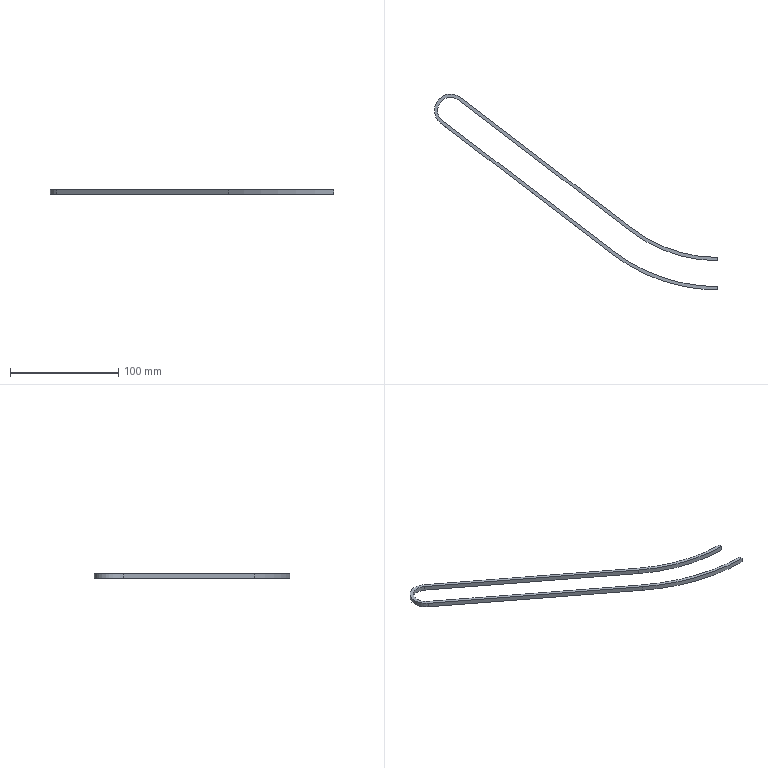Part | STEP file | 1 solid | 15 faces | box 261.956 x 181.154 x 4 mm | volume 7579 mm3 | plane 8 | cylinder 7 | commonest cylinder face diameters 24 x2 30 x1 260 x1 266 x1 314 x1 320 x1
STEP:
#1=CARTESIAN_POINT('',(0.,0.,0.));
#2=DIRECTION('',(0.,0.,1.));
#3=DIRECTION('',(1.,0.,0.));
#4=AXIS2_PLACEMENT_3D('',#1,#2,#3);
#5=CARTESIAN_POINT('',(-78.156,99.707,0.));
#6=VERTEX_POINT('',#5);
#7=CARTESIAN_POINT('',(-78.156,99.707,4.));
#8=VERTEX_POINT('',#7);
#9=CARTESIAN_POINT('',(-78.156,99.707,4.));
#10=DIRECTION('',(0.,0.,1.));
#11=VECTOR('',#10,1.);
#12=LINE('',#9,#11);
#13=CARTESIAN_POINT('',(-85.439,90.17,4.));
#14=DIRECTION('',(0.,0.,-1.));
#15=DIRECTION('',(-1.,0.,0.));
#16=AXIS2_PLACEMENT_3D('',#13,#14,#15);
#17=CYLINDRICAL_SURFACE('',#16,12.);
#18=CARTESIAN_POINT('',(2.223,0.));
#19=DIRECTION('',(0.,-1.));
#20=VECTOR('',#19,1.);
#21=LINE('',#18,#20);
#22=(GEOMETRIC_REPRESENTATION_CONTEXT(2)PARAMETRIC_REPRESENTATION_CONTEXT()REPRESENTATION_CONTEXT('',''));
#23=DEFINITIONAL_REPRESENTATION('',(#21),#22);
#24=PCURVE('',#17,#23);
#25=CARTESIAN_POINT('',(-78.156,99.707,4.));
#26=DIRECTION('',(0.607,0.7947,0.));
#27=DIRECTION('',(-0.7947,0.607,0.));
#28=AXIS2_PLACEMENT_3D('',#25,#26,#27);
#29=PLANE('',#28);
#30=CARTESIAN_POINT('',(0.,0.));
#31=DIRECTION('',(0.,1.));
#32=VECTOR('',#31,1.);
#33=LINE('',#30,#32);
#34=(GEOMETRIC_REPRESENTATION_CONTEXT(2)PARAMETRIC_REPRESENTATION_CONTEXT()REPRESENTATION_CONTEXT('',''));
#35=DEFINITIONAL_REPRESENTATION('',(#33),#34);
#36=PCURVE('',#29,#35);
#37=SURFACE_CURVE('',#12,(#24,#36),.PCURVE_S1.);
#38=EDGE_CURVE('',#6,#8,#37,.T.);
#39=ORIENTED_EDGE('',*,*,#38,.F.);
#40=CARTESIAN_POINT('',(-97.439,90.17,0.));
#41=VERTEX_POINT('',#40);
#42=CARTESIAN_POINT('',(-85.439,90.17,0.));
#43=DIRECTION('',(0.,0.,1.));
#44=DIRECTION('',(-1.,0.,0.));
#45=AXIS2_PLACEMENT_3D('',#42,#43,#44);
#46=CIRCLE('',#45,12.);
#47=CARTESIAN_POINT('',(6.283,4.));
#48=DIRECTION('',(-1.,0.));
#49=VECTOR('',#48,1.);
#50=LINE('',#47,#49);
#51=(GEOMETRIC_REPRESENTATION_CONTEXT(2)PARAMETRIC_REPRESENTATION_CONTEXT()REPRESENTATION_CONTEXT('',''));
#52=DEFINITIONAL_REPRESENTATION('',(#50),#51);
#53=PCURVE('',#17,#52);
#54=CARTESIAN_POINT('',(25.595,9.755,0.));
#55=DIRECTION('',(0.,0.,1.));
#56=DIRECTION('',(1.,0.,0.));
#57=AXIS2_PLACEMENT_3D('',#54,#55,#56);
#58=PLANE('',#57);
#59=CARTESIAN_POINT('',(-111.034,80.414));
#60=DIRECTION('',(-1.,0.));
#61=AXIS2_PLACEMENT_2D('',#59,#60);
#62=CIRCLE('',#61,12.);
#63=(GEOMETRIC_REPRESENTATION_CONTEXT(2)PARAMETRIC_REPRESENTATION_CONTEXT()REPRESENTATION_CONTEXT('',''));
#64=DEFINITIONAL_REPRESENTATION('',(#62),#63);
#65=PCURVE('',#58,#64);
#66=SURFACE_CURVE('',#46,(#53,#65),.PCURVE_S1.);
#67=EDGE_CURVE('',#6,#41,#66,.T.);
#68=ORIENTED_EDGE('',*,*,#67,.T.);
#69=CARTESIAN_POINT('',(-97.439,90.17,4.));
#70=VERTEX_POINT('',#69);
#71=CARTESIAN_POINT('',(-97.439,90.17,4.));
#72=DIRECTION('',(0.,0.,-1.));
#73=VECTOR('',#72,1.);
#74=LINE('',#71,#73);
#75=CARTESIAN_POINT('',(0.,0.));
#76=DIRECTION('',(0.,1.));
#77=VECTOR('',#76,1.);
#78=LINE('',#75,#77);
#79=(GEOMETRIC_REPRESENTATION_CONTEXT(2)PARAMETRIC_REPRESENTATION_CONTEXT()REPRESENTATION_CONTEXT('',''));
#80=DEFINITIONAL_REPRESENTATION('',(#78),#79);
#81=PCURVE('',#17,#80);
#82=CARTESIAN_POINT('',(-85.439,90.17,4.));
#83=DIRECTION('',(0.,0.,-1.));
#84=DIRECTION('',(-1.,0.,0.));
#85=AXIS2_PLACEMENT_3D('',#82,#83,#84);
#86=CYLINDRICAL_SURFACE('',#85,12.);
#87=CARTESIAN_POINT('',(6.283,0.));
#88=DIRECTION('',(0.,1.));
#89=VECTOR('',#88,1.);
#90=LINE('',#87,#89);
#91=(GEOMETRIC_REPRESENTATION_CONTEXT(2)PARAMETRIC_REPRESENTATION_CONTEXT()REPRESENTATION_CONTEXT('',''));
#92=DEFINITIONAL_REPRESENTATION('',(#90),#91);
#93=PCURVE('',#86,#92);
#94=SURFACE_CURVE('',#74,(#81,#93),.PCURVE_S1.);
#95=EDGE_CURVE('',#70,#41,#94,.T.);
#96=ORIENTED_EDGE('',*,*,#95,.F.);
#97=CARTESIAN_POINT('',(-85.439,90.17,4.));
#98=DIRECTION('',(0.,0.,-1.));
#99=DIRECTION('',(-1.,0.,0.));
#100=AXIS2_PLACEMENT_3D('',#97,#98,#99);
#101=CIRCLE('',#100,12.);
#102=CARTESIAN_POINT('',(0.,0.));
#103=DIRECTION('',(1.,0.));
#104=VECTOR('',#103,1.);
#105=LINE('',#102,#104);
#106=(GEOMETRIC_REPRESENTATION_CONTEXT(2)PARAMETRIC_REPRESENTATION_CONTEXT()REPRESENTATION_CONTEXT('',''));
#107=DEFINITIONAL_REPRESENTATION('',(#105),#106);
#108=PCURVE('',#17,#107);
#109=CARTESIAN_POINT('',(25.595,9.755,4.));
#110=DIRECTION('',(0.,0.,1.));
#111=DIRECTION('',(1.,0.,0.));
#112=AXIS2_PLACEMENT_3D('',#109,#110,#111);
#113=PLANE('',#112);
#114=CARTESIAN_POINT('',(-123.034,80.414));
#115=CARTESIAN_POINT('',(-123.034,101.199));
#116=CARTESIAN_POINT('',(-105.034,90.807));
#117=CARTESIAN_POINT('',(-87.034,80.414));
#118=CARTESIAN_POINT('',(-105.034,70.022));
#119=CARTESIAN_POINT('',(-123.034,59.63));
#120=CARTESIAN_POINT('',(-123.034,80.414));
#121=(BOUNDED_CURVE()B_SPLINE_CURVE(2,(#114,#115,#116,#117,#118,#119,#120),.UNSPECIFIED.,.T.,.F.)B_SPLINE_CURVE_WITH_KNOTS((1,2,2,2,2,1),(-2.094,0.,2.094,4.189,6.283,8.378),.UNSPECIFIED.)CURVE()GEOMETRIC_REPRESENTATION_ITEM()RATIONAL_B_SPLINE_CURVE((1.,0.5,1.,0.5,1.,0.5,1.))REPRESENTATION_ITEM(''));
#122=(GEOMETRIC_REPRESENTATION_CONTEXT(2)PARAMETRIC_REPRESENTATION_CONTEXT()REPRESENTATION_CONTEXT('',''));
#123=DEFINITIONAL_REPRESENTATION('',(#121),#122);
#124=PCURVE('',#113,#123);
#125=SURFACE_CURVE('',#101,(#108,#124),.PCURVE_S1.);
#126=EDGE_CURVE('',#70,#8,#125,.T.);
#127=ORIENTED_EDGE('',*,*,#126,.T.);
#128=EDGE_LOOP('',(#39,#68,#96,#127));
#129=FACE_BOUND('',#128,.F.);
#130=ADVANCED_FACE('',(#129),#17,.F.);
#131=CARTESIAN_POINT('',(-92.723,80.633,4.));
#132=VERTEX_POINT('',#131);
#133=CARTESIAN_POINT('',(-85.439,90.17,4.));
#134=DIRECTION('',(0.,0.,-1.));
#135=DIRECTION('',(-1.,0.,0.));
#136=AXIS2_PLACEMENT_3D('',#133,#134,#135);
#137=CIRCLE('',#136,12.);
#138=CARTESIAN_POINT('',(-123.034,80.414));
#139=CARTESIAN_POINT('',(-123.034,101.199));
#140=CARTESIAN_POINT('',(-105.034,90.807));
#141=CARTESIAN_POINT('',(-87.034,80.414));
#142=CARTESIAN_POINT('',(-105.034,70.022));
#143=CARTESIAN_POINT('',(-123.034,59.63));
#144=CARTESIAN_POINT('',(-123.034,80.414));
#145=(BOUNDED_CURVE()B_SPLINE_CURVE(2,(#138,#139,#140,#141,#142,#143,#144),.UNSPECIFIED.,.T.,.F.)B_SPLINE_CURVE_WITH_KNOTS((1,2,2,2,2,1),(-2.094,0.,2.094,4.189,6.283,8.378),.UNSPECIFIED.)CURVE()GEOMETRIC_REPRESENTATION_ITEM()RATIONAL_B_SPLINE_CURVE((1.,0.5,1.,0.5,1.,0.5,1.))REPRESENTATION_ITEM(''));
#146=(GEOMETRIC_REPRESENTATION_CONTEXT(2)PARAMETRIC_REPRESENTATION_CONTEXT()REPRESENTATION_CONTEXT('',''));
#147=DEFINITIONAL_REPRESENTATION('',(#145),#146);
#148=PCURVE('',#113,#147);
#149=CARTESIAN_POINT('',(0.,0.));
#150=DIRECTION('',(1.,0.));
#151=VECTOR('',#150,1.);
#152=LINE('',#149,#151);
#153=(GEOMETRIC_REPRESENTATION_CONTEXT(2)PARAMETRIC_REPRESENTATION_CONTEXT()REPRESENTATION_CONTEXT('',''));
#154=DEFINITIONAL_REPRESENTATION('',(#152),#153);
#155=PCURVE('',#86,#154);
#156=SURFACE_CURVE('',#137,(#148,#155),.PCURVE_S1.);
#157=EDGE_CURVE('',#132,#70,#156,.T.);
#158=ORIENTED_EDGE('',*,*,#157,.T.);
#159=ORIENTED_EDGE('',*,*,#126,.T.);
#160=CARTESIAN_POINT('',(80.791,-21.684,4.));
#161=VERTEX_POINT('',#160);
#162=CARTESIAN_POINT('',(-78.156,99.707,4.));
#163=DIRECTION('',(0.7947,-0.607,0.));
#164=VECTOR('',#163,1.);
#165=LINE('',#162,#164);
#166=CARTESIAN_POINT('',(-103.75,89.951));
#167=DIRECTION('',(0.7947,-0.607));
#168=VECTOR('',#167,1.);
#169=LINE('',#166,#168);
#170=(GEOMETRIC_REPRESENTATION_CONTEXT(2)PARAMETRIC_REPRESENTATION_CONTEXT()REPRESENTATION_CONTEXT('',''));
#171=DEFINITIONAL_REPRESENTATION('',(#169),#170);
#172=PCURVE('',#113,#171);
#173=CARTESIAN_POINT('',(0.,0.));
#174=DIRECTION('',(-1.,0.));
#175=VECTOR('',#174,1.);
#176=LINE('',#173,#175);
#177=(GEOMETRIC_REPRESENTATION_CONTEXT(2)PARAMETRIC_REPRESENTATION_CONTEXT()REPRESENTATION_CONTEXT('',''));
#178=DEFINITIONAL_REPRESENTATION('',(#176),#177);
#179=PCURVE('',#29,#178);
#180=SURFACE_CURVE('',#165,(#172,#179),.PCURVE_S1.);
#181=EDGE_CURVE('',#8,#161,#180,.T.);
#182=ORIENTED_EDGE('',*,*,#181,.T.);
#183=CARTESIAN_POINT('',(161.516,-48.985,4.));
#184=VERTEX_POINT('',#183);
#185=CARTESIAN_POINT('',(161.516,84.015,4.));
#186=DIRECTION('',(0.,0.,1.));
#187=DIRECTION('',(-1.,0.,0.));
#188=AXIS2_PLACEMENT_3D('',#185,#186,#187);
#189=CIRCLE('',#188,133.);
#190=CARTESIAN_POINT('',(135.922,74.26));
#191=DIRECTION('',(-1.,0.));
#192=AXIS2_PLACEMENT_2D('',#190,#191);
#193=CIRCLE('',#192,133.);
#194=(GEOMETRIC_REPRESENTATION_CONTEXT(2)PARAMETRIC_REPRESENTATION_CONTEXT()REPRESENTATION_CONTEXT('',''));
#195=DEFINITIONAL_REPRESENTATION('',(#193),#194);
#196=PCURVE('',#113,#195);
#197=CARTESIAN_POINT('',(161.516,84.015,4.));
#198=DIRECTION('',(0.,0.,-1.));
#199=DIRECTION('',(-1.,0.,0.));
#200=AXIS2_PLACEMENT_3D('',#197,#198,#199);
#201=CYLINDRICAL_SURFACE('',#200,133.);
#202=CARTESIAN_POINT('',(6.283,0.));
#203=DIRECTION('',(-1.,0.));
#204=VECTOR('',#203,1.);
#205=LINE('',#202,#204);
#206=(GEOMETRIC_REPRESENTATION_CONTEXT(2)PARAMETRIC_REPRESENTATION_CONTEXT()REPRESENTATION_CONTEXT('',''));
#207=DEFINITIONAL_REPRESENTATION('',(#205),#206);
#208=PCURVE('',#201,#207);
#209=SURFACE_CURVE('',#189,(#196,#208),.PCURVE_S1.);
#210=EDGE_CURVE('',#161,#184,#209,.T.);
#211=ORIENTED_EDGE('',*,*,#210,.T.);
#212=CARTESIAN_POINT('',(161.516,-45.985,4.));
#213=VERTEX_POINT('',#212);
#214=CARTESIAN_POINT('',(161.516,9.755,4.));
#215=DIRECTION('',(0.,1.,0.));
#216=VECTOR('',#215,1.);
#217=LINE('',#214,#216);
#218=CARTESIAN_POINT('',(135.922,0.));
#219=DIRECTION('',(0.,1.));
#220=VECTOR('',#219,1.);
#221=LINE('',#218,#220);
#222=(GEOMETRIC_REPRESENTATION_CONTEXT(2)PARAMETRIC_REPRESENTATION_CONTEXT()REPRESENTATION_CONTEXT('',''));
#223=DEFINITIONAL_REPRESENTATION('',(#221),#222);
#224=PCURVE('',#113,#223);
#225=CARTESIAN_POINT('',(161.516,-75.985,0.));
#226=DIRECTION('',(1.,0.,0.));
#227=DIRECTION('',(0.,0.,-1.));
#228=AXIS2_PLACEMENT_3D('',#225,#226,#227);
#229=PLANE('',#228);
#230=CARTESIAN_POINT('',(-4.,85.74));
#231=DIRECTION('',(0.,1.));
#232=VECTOR('',#231,1.);
#233=LINE('',#230,#232);
#234=(GEOMETRIC_REPRESENTATION_CONTEXT(2)PARAMETRIC_REPRESENTATION_CONTEXT()REPRESENTATION_CONTEXT('',''));
#235=DEFINITIONAL_REPRESENTATION('',(#233),#234);
#236=PCURVE('',#229,#235);
#237=SURFACE_CURVE('',#217,(#224,#236),.PCURVE_S1.);
#238=EDGE_CURVE('',#184,#213,#237,.T.);
#239=ORIENTED_EDGE('',*,*,#238,.T.);
#240=CARTESIAN_POINT('',(82.612,-19.3,4.));
#241=VERTEX_POINT('',#240);
#242=CARTESIAN_POINT('',(161.516,84.015,4.));
#243=DIRECTION('',(0.,0.,-1.));
#244=DIRECTION('',(1.,0.,0.));
#245=AXIS2_PLACEMENT_3D('',#242,#243,#244);
#246=CIRCLE('',#245,130.);
#247=CARTESIAN_POINT('',(265.922,74.26));
#248=CARTESIAN_POINT('',(265.922,-150.907));
#249=CARTESIAN_POINT('',(70.922,-38.323));
#250=CARTESIAN_POINT('',(-124.078,74.26));
#251=CARTESIAN_POINT('',(70.922,186.843));
#252=CARTESIAN_POINT('',(265.922,299.427));
#253=CARTESIAN_POINT('',(265.922,74.26));
#254=(BOUNDED_CURVE()B_SPLINE_CURVE(2,(#247,#248,#249,#250,#251,#252,#253),.UNSPECIFIED.,.T.,.F.)B_SPLINE_CURVE_WITH_KNOTS((1,2,2,2,2,1),(-2.094,0.,2.094,4.189,6.283,8.378),.UNSPECIFIED.)CURVE()GEOMETRIC_REPRESENTATION_ITEM()RATIONAL_B_SPLINE_CURVE((1.,0.5,1.,0.5,1.,0.5,1.))REPRESENTATION_ITEM(''));
#255=(GEOMETRIC_REPRESENTATION_CONTEXT(2)PARAMETRIC_REPRESENTATION_CONTEXT()REPRESENTATION_CONTEXT('',''));
#256=DEFINITIONAL_REPRESENTATION('',(#254),#255);
#257=PCURVE('',#113,#256);
#258=CARTESIAN_POINT('',(161.516,84.015,0.));
#259=DIRECTION('',(0.,0.,1.));
#260=DIRECTION('',(1.,0.,0.));
#261=AXIS2_PLACEMENT_3D('',#258,#259,#260);
#262=CYLINDRICAL_SURFACE('',#261,130.);
#263=CARTESIAN_POINT('',(6.283,4.));
#264=DIRECTION('',(-1.,0.));
#265=VECTOR('',#264,1.);
#266=LINE('',#263,#265);
#267=(GEOMETRIC_REPRESENTATION_CONTEXT(2)PARAMETRIC_REPRESENTATION_CONTEXT()REPRESENTATION_CONTEXT('',''));
#268=DEFINITIONAL_REPRESENTATION('',(#266),#267);
#269=PCURVE('',#262,#268);
#270=SURFACE_CURVE('',#246,(#257,#269),.PCURVE_S1.);
#271=EDGE_CURVE('',#213,#241,#270,.T.);
#272=ORIENTED_EDGE('',*,*,#271,.T.);
#273=CARTESIAN_POINT('',(-76.335,102.091,4.));
#274=VERTEX_POINT('',#273);
#275=CARTESIAN_POINT('',(82.612,-19.3,4.));
#276=DIRECTION('',(-0.7947,0.607,0.));
#277=VECTOR('',#276,1.);
#278=LINE('',#275,#277);
#279=CARTESIAN_POINT('',(57.018,-29.056));
#280=DIRECTION('',(-0.7947,0.607));
#281=VECTOR('',#280,1.);
#282=LINE('',#279,#281);
#283=(GEOMETRIC_REPRESENTATION_CONTEXT(2)PARAMETRIC_REPRESENTATION_CONTEXT()REPRESENTATION_CONTEXT('',''));
#284=DEFINITIONAL_REPRESENTATION('',(#282),#283);
#285=PCURVE('',#113,#284);
#286=CARTESIAN_POINT('',(82.612,-19.3,0.));
#287=DIRECTION('',(0.607,0.7947,0.));
#288=DIRECTION('',(-0.7947,0.607,0.));
#289=AXIS2_PLACEMENT_3D('',#286,#287,#288);
#290=PLANE('',#289);
#291=CARTESIAN_POINT('',(0.,4.));
#292=DIRECTION('',(1.,0.));
#293=VECTOR('',#292,1.);
#294=LINE('',#291,#293);
#295=(GEOMETRIC_REPRESENTATION_CONTEXT(2)PARAMETRIC_REPRESENTATION_CONTEXT()REPRESENTATION_CONTEXT('',''));
#296=DEFINITIONAL_REPRESENTATION('',(#294),#295);
#297=PCURVE('',#290,#296);
#298=SURFACE_CURVE('',#278,(#285,#297),.PCURVE_S1.);
#299=EDGE_CURVE('',#241,#274,#298,.T.);
#300=ORIENTED_EDGE('',*,*,#299,.T.);
#301=CARTESIAN_POINT('',(-94.544,78.249,4.));
#302=VERTEX_POINT('',#301);
#303=CARTESIAN_POINT('',(-85.439,90.17,4.));
#304=DIRECTION('',(0.,0.,1.));
#305=DIRECTION('',(1.,0.,0.));
#306=AXIS2_PLACEMENT_3D('',#303,#304,#305);
#307=CIRCLE('',#306,15.);
#308=CARTESIAN_POINT('',(-111.034,80.414));
#309=DIRECTION('',(1.,0.));
#310=AXIS2_PLACEMENT_2D('',#308,#309);
#311=CIRCLE('',#310,15.);
#312=(GEOMETRIC_REPRESENTATION_CONTEXT(2)PARAMETRIC_REPRESENTATION_CONTEXT()REPRESENTATION_CONTEXT('',''));
#313=DEFINITIONAL_REPRESENTATION('',(#311),#312);
#314=PCURVE('',#113,#313);
#315=CARTESIAN_POINT('',(-85.439,90.17,0.));
#316=DIRECTION('',(0.,0.,1.));
#317=DIRECTION('',(1.,0.,0.));
#318=AXIS2_PLACEMENT_3D('',#315,#316,#317);
#319=CYLINDRICAL_SURFACE('',#318,15.);
#320=CARTESIAN_POINT('',(0.,4.));
#321=DIRECTION('',(1.,0.));
#322=VECTOR('',#321,1.);
#323=LINE('',#320,#322);
#324=(GEOMETRIC_REPRESENTATION_CONTEXT(2)PARAMETRIC_REPRESENTATION_CONTEXT()REPRESENTATION_CONTEXT('',''));
#325=DEFINITIONAL_REPRESENTATION('',(#323),#324);
#326=PCURVE('',#319,#325);
#327=SURFACE_CURVE('',#307,(#314,#326),.PCURVE_S1.);
#328=EDGE_CURVE('',#274,#302,#327,.T.);
#329=ORIENTED_EDGE('',*,*,#328,.T.);
#330=CARTESIAN_POINT('',(64.404,-43.142,4.));
#331=VERTEX_POINT('',#330);
#332=CARTESIAN_POINT('',(-94.544,78.249,4.));
#333=DIRECTION('',(0.7947,-0.607,0.));
#334=VECTOR('',#333,1.);
#335=LINE('',#332,#334);
#336=CARTESIAN_POINT('',(-120.138,68.493));
#337=DIRECTION('',(0.7947,-0.607));
#338=VECTOR('',#337,1.);
#339=LINE('',#336,#338);
#340=(GEOMETRIC_REPRESENTATION_CONTEXT(2)PARAMETRIC_REPRESENTATION_CONTEXT()REPRESENTATION_CONTEXT('',''));
#341=DEFINITIONAL_REPRESENTATION('',(#339),#340);
#342=PCURVE('',#113,#341);
#343=CARTESIAN_POINT('',(-94.544,78.249,0.));
#344=DIRECTION('',(-0.607,-0.7947,0.));
#345=DIRECTION('',(0.7947,-0.607,0.));
#346=AXIS2_PLACEMENT_3D('',#343,#344,#345);
#347=PLANE('',#346);
#348=CARTESIAN_POINT('',(0.,4.));
#349=DIRECTION('',(1.,0.));
#350=VECTOR('',#349,1.);
#351=LINE('',#348,#350);
#352=(GEOMETRIC_REPRESENTATION_CONTEXT(2)PARAMETRIC_REPRESENTATION_CONTEXT()REPRESENTATION_CONTEXT('',''));
#353=DEFINITIONAL_REPRESENTATION('',(#351),#352);
#354=PCURVE('',#347,#353);
#355=SURFACE_CURVE('',#335,(#342,#354),.PCURVE_S1.);
#356=EDGE_CURVE('',#302,#331,#355,.T.);
#357=ORIENTED_EDGE('',*,*,#356,.T.);
#358=CARTESIAN_POINT('',(161.516,-75.985,4.));
#359=VERTEX_POINT('',#358);
#360=CARTESIAN_POINT('',(161.516,84.015,4.));
#361=DIRECTION('',(0.,0.,1.));
#362=DIRECTION('',(1.,0.,0.));
#363=AXIS2_PLACEMENT_3D('',#360,#361,#362);
#364=CIRCLE('',#363,160.);
#365=CARTESIAN_POINT('',(135.922,74.26));
#366=DIRECTION('',(1.,0.));
#367=AXIS2_PLACEMENT_2D('',#365,#366);
#368=CIRCLE('',#367,160.);
#369=(GEOMETRIC_REPRESENTATION_CONTEXT(2)PARAMETRIC_REPRESENTATION_CONTEXT()REPRESENTATION_CONTEXT('',''));
#370=DEFINITIONAL_REPRESENTATION('',(#368),#369);
#371=PCURVE('',#113,#370);
#372=CARTESIAN_POINT('',(161.516,84.015,0.));
#373=DIRECTION('',(0.,0.,1.));
#374=DIRECTION('',(1.,0.,0.));
#375=AXIS2_PLACEMENT_3D('',#372,#373,#374);
#376=CYLINDRICAL_SURFACE('',#375,160.);
#377=CARTESIAN_POINT('',(0.,4.));
#378=DIRECTION('',(1.,0.));
#379=VECTOR('',#378,1.);
#380=LINE('',#377,#379);
#381=(GEOMETRIC_REPRESENTATION_CONTEXT(2)PARAMETRIC_REPRESENTATION_CONTEXT()REPRESENTATION_CONTEXT('',''));
#382=DEFINITIONAL_REPRESENTATION('',(#380),#381);
#383=PCURVE('',#376,#382);
#384=SURFACE_CURVE('',#364,(#371,#383),.PCURVE_S1.);
#385=EDGE_CURVE('',#331,#359,#384,.T.);
#386=ORIENTED_EDGE('',*,*,#385,.T.);
#387=CARTESIAN_POINT('',(161.516,-72.985,4.));
#388=VERTEX_POINT('',#387);
#389=CARTESIAN_POINT('',(161.516,9.755,4.));
#390=DIRECTION('',(0.,1.,0.));
#391=VECTOR('',#390,1.);
#392=LINE('',#389,#391);
#393=CARTESIAN_POINT('',(135.922,0.));
#394=DIRECTION('',(0.,1.));
#395=VECTOR('',#394,1.);
#396=LINE('',#393,#395);
#397=(GEOMETRIC_REPRESENTATION_CONTEXT(2)PARAMETRIC_REPRESENTATION_CONTEXT()REPRESENTATION_CONTEXT('',''));
#398=DEFINITIONAL_REPRESENTATION('',(#396),#397);
#399=PCURVE('',#113,#398);
#400=CARTESIAN_POINT('',(161.516,-75.985,0.));
#401=DIRECTION('',(1.,0.,0.));
#402=DIRECTION('',(0.,0.,-1.));
#403=AXIS2_PLACEMENT_3D('',#400,#401,#402);
#404=PLANE('',#403);
#405=CARTESIAN_POINT('',(-4.,85.74));
#406=DIRECTION('',(0.,1.));
#407=VECTOR('',#406,1.);
#408=LINE('',#405,#407);
#409=(GEOMETRIC_REPRESENTATION_CONTEXT(2)PARAMETRIC_REPRESENTATION_CONTEXT()REPRESENTATION_CONTEXT('',''));
#410=DEFINITIONAL_REPRESENTATION('',(#408),#409);
#411=PCURVE('',#404,#410);
#412=SURFACE_CURVE('',#392,(#399,#411),.PCURVE_S1.);
#413=EDGE_CURVE('',#359,#388,#412,.T.);
#414=ORIENTED_EDGE('',*,*,#413,.T.);
#415=CARTESIAN_POINT('',(66.224,-40.758,4.));
#416=VERTEX_POINT('',#415);
#417=CARTESIAN_POINT('',(161.516,84.015,4.));
#418=DIRECTION('',(0.,0.,-1.));
#419=DIRECTION('',(-1.,0.,0.));
#420=AXIS2_PLACEMENT_3D('',#417,#418,#419);
#421=CIRCLE('',#420,157.);
#422=CARTESIAN_POINT('',(-21.078,74.26));
#423=CARTESIAN_POINT('',(-21.078,346.192));
#424=CARTESIAN_POINT('',(214.422,210.226));
#425=CARTESIAN_POINT('',(449.922,74.26));
#426=CARTESIAN_POINT('',(214.422,-61.706));
#427=CARTESIAN_POINT('',(-21.078,-197.672));
#428=CARTESIAN_POINT('',(-21.078,74.26));
#429=(BOUNDED_CURVE()B_SPLINE_CURVE(2,(#422,#423,#424,#425,#426,#427,#428),.UNSPECIFIED.,.T.,.F.)B_SPLINE_CURVE_WITH_KNOTS((1,2,2,2,2,1),(-2.094,0.,2.094,4.189,6.283,8.378),.UNSPECIFIED.)CURVE()GEOMETRIC_REPRESENTATION_ITEM()RATIONAL_B_SPLINE_CURVE((1.,0.5,1.,0.5,1.,0.5,1.))REPRESENTATION_ITEM(''));
#430=(GEOMETRIC_REPRESENTATION_CONTEXT(2)PARAMETRIC_REPRESENTATION_CONTEXT()REPRESENTATION_CONTEXT('',''));
#431=DEFINITIONAL_REPRESENTATION('',(#429),#430);
#432=PCURVE('',#113,#431);
#433=CARTESIAN_POINT('',(161.516,84.015,4.));
#434=DIRECTION('',(0.,0.,-1.));
#435=DIRECTION('',(-1.,0.,0.));
#436=AXIS2_PLACEMENT_3D('',#433,#434,#435);
#437=CYLINDRICAL_SURFACE('',#436,157.);
#438=CARTESIAN_POINT('',(0.,0.));
#439=DIRECTION('',(1.,0.));
#440=VECTOR('',#439,1.);
#441=LINE('',#438,#440);
#442=(GEOMETRIC_REPRESENTATION_CONTEXT(2)PARAMETRIC_REPRESENTATION_CONTEXT()REPRESENTATION_CONTEXT('',''));
#443=DEFINITIONAL_REPRESENTATION('',(#441),#442);
#444=PCURVE('',#437,#443);
#445=SURFACE_CURVE('',#421,(#432,#444),.PCURVE_S1.);
#446=EDGE_CURVE('',#388,#416,#445,.T.);
#447=ORIENTED_EDGE('',*,*,#446,.T.);
#448=CARTESIAN_POINT('',(66.224,-40.758,4.));
#449=DIRECTION('',(-0.7947,0.607,0.));
#450=VECTOR('',#449,1.);
#451=LINE('',#448,#450);
#452=CARTESIAN_POINT('',(40.63,-50.514));
#453=DIRECTION('',(-0.7947,0.607));
#454=VECTOR('',#453,1.);
#455=LINE('',#452,#454);
#456=(GEOMETRIC_REPRESENTATION_CONTEXT(2)PARAMETRIC_REPRESENTATION_CONTEXT()REPRESENTATION_CONTEXT('',''));
#457=DEFINITIONAL_REPRESENTATION('',(#455),#456);
#458=PCURVE('',#113,#457);
#459=CARTESIAN_POINT('',(66.224,-40.758,4.));
#460=DIRECTION('',(-0.607,-0.7947,0.));
#461=DIRECTION('',(0.7947,-0.607,0.));
#462=AXIS2_PLACEMENT_3D('',#459,#460,#461);
#463=PLANE('',#462);
#464=CARTESIAN_POINT('',(0.,0.));
#465=DIRECTION('',(-1.,0.));
#466=VECTOR('',#465,1.);
#467=LINE('',#464,#466);
#468=(GEOMETRIC_REPRESENTATION_CONTEXT(2)PARAMETRIC_REPRESENTATION_CONTEXT()REPRESENTATION_CONTEXT('',''));
#469=DEFINITIONAL_REPRESENTATION('',(#467),#468);
#470=PCURVE('',#463,#469);
#471=SURFACE_CURVE('',#451,(#458,#470),.PCURVE_S1.);
#472=EDGE_CURVE('',#416,#132,#471,.T.);
#473=ORIENTED_EDGE('',*,*,#472,.T.);
#474=EDGE_LOOP('',(#158,#159,#182,#211,#239,#272,#300,#329,#357,#386,#414,#447,#473));
#475=FACE_BOUND('',#474,.T.);
#476=ADVANCED_FACE('',(#475),#113,.T.);
#477=CARTESIAN_POINT('',(80.791,-21.684,0.));
#478=VERTEX_POINT('',#477);
#479=CARTESIAN_POINT('',(80.791,-21.684,4.));
#480=DIRECTION('',(0.,0.,-1.));
#481=VECTOR('',#480,1.);
#482=LINE('',#479,#481);
#483=CARTESIAN_POINT('',(-200.,0.));
#484=DIRECTION('',(0.,-1.));
#485=VECTOR('',#484,1.);
#486=LINE('',#483,#485);
#487=(GEOMETRIC_REPRESENTATION_CONTEXT(2)PARAMETRIC_REPRESENTATION_CONTEXT()REPRESENTATION_CONTEXT('',''));
#488=DEFINITIONAL_REPRESENTATION('',(#486),#487);
#489=PCURVE('',#29,#488);
#490=CARTESIAN_POINT('',(5.365,0.));
#491=DIRECTION('',(0.,1.));
#492=VECTOR('',#491,1.);
#493=LINE('',#490,#492);
#494=(GEOMETRIC_REPRESENTATION_CONTEXT(2)PARAMETRIC_REPRESENTATION_CONTEXT()REPRESENTATION_CONTEXT('',''));
#495=DEFINITIONAL_REPRESENTATION('',(#493),#494);
#496=PCURVE('',#201,#495);
#497=SURFACE_CURVE('',#482,(#489,#496),.PCURVE_S1.);
#498=EDGE_CURVE('',#161,#478,#497,.T.);
#499=ORIENTED_EDGE('',*,*,#498,.F.);
#500=ORIENTED_EDGE('',*,*,#181,.F.);
#501=ORIENTED_EDGE('',*,*,#38,.F.);
#502=CARTESIAN_POINT('',(-78.156,99.707,0.));
#503=DIRECTION('',(-0.7947,0.607,0.));
#504=VECTOR('',#503,1.);
#505=LINE('',#502,#504);
#506=CARTESIAN_POINT('',(0.,-4.));
#507=DIRECTION('',(1.,0.));
#508=VECTOR('',#507,1.);
#509=LINE('',#506,#508);
#510=(GEOMETRIC_REPRESENTATION_CONTEXT(2)PARAMETRIC_REPRESENTATION_CONTEXT()REPRESENTATION_CONTEXT('',''));
#511=DEFINITIONAL_REPRESENTATION('',(#509),#510);
#512=PCURVE('',#29,#511);
#513=CARTESIAN_POINT('',(-103.75,89.951));
#514=DIRECTION('',(-0.7947,0.607));
#515=VECTOR('',#514,1.);
#516=LINE('',#513,#515);
#517=(GEOMETRIC_REPRESENTATION_CONTEXT(2)PARAMETRIC_REPRESENTATION_CONTEXT()REPRESENTATION_CONTEXT('',''));
#518=DEFINITIONAL_REPRESENTATION('',(#516),#517);
#519=PCURVE('',#58,#518);
#520=SURFACE_CURVE('',#505,(#512,#519),.PCURVE_S1.);
#521=EDGE_CURVE('',#478,#6,#520,.T.);
#522=ORIENTED_EDGE('',*,*,#521,.F.);
#523=EDGE_LOOP('',(#499,#500,#501,#522));
#524=FACE_BOUND('',#523,.T.);
#525=ADVANCED_FACE('',(#524),#29,.F.);
#526=CARTESIAN_POINT('',(-92.723,80.633,0.));
#527=VERTEX_POINT('',#526);
#528=CARTESIAN_POINT('',(-85.439,90.17,0.));
#529=DIRECTION('',(0.,0.,1.));
#530=DIRECTION('',(-1.,0.,0.));
#531=AXIS2_PLACEMENT_3D('',#528,#529,#530);
#532=CIRCLE('',#531,12.);
#533=CARTESIAN_POINT('',(6.283,4.));
#534=DIRECTION('',(-1.,0.));
#535=VECTOR('',#534,1.);
#536=LINE('',#533,#535);
#537=(GEOMETRIC_REPRESENTATION_CONTEXT(2)PARAMETRIC_REPRESENTATION_CONTEXT()REPRESENTATION_CONTEXT('',''));
#538=DEFINITIONAL_REPRESENTATION('',(#536),#537);
#539=PCURVE('',#86,#538);
#540=CARTESIAN_POINT('',(-111.034,80.414));
#541=DIRECTION('',(-1.,0.));
#542=AXIS2_PLACEMENT_2D('',#540,#541);
#543=CIRCLE('',#542,12.);
#544=(GEOMETRIC_REPRESENTATION_CONTEXT(2)PARAMETRIC_REPRESENTATION_CONTEXT()REPRESENTATION_CONTEXT('',''));
#545=DEFINITIONAL_REPRESENTATION('',(#543),#544);
#546=PCURVE('',#58,#545);
#547=SURFACE_CURVE('',#532,(#539,#546),.PCURVE_S1.);
#548=EDGE_CURVE('',#41,#527,#547,.T.);
#549=ORIENTED_EDGE('',*,*,#548,.T.);
#550=CARTESIAN_POINT('',(-92.723,80.633,4.));
#551=DIRECTION('',(0.,0.,1.));
#552=VECTOR('',#551,1.);
#553=LINE('',#550,#552);
#554=CARTESIAN_POINT('',(5.365,0.));
#555=DIRECTION('',(0.,-1.));
#556=VECTOR('',#555,1.);
#557=LINE('',#554,#556);
#558=(GEOMETRIC_REPRESENTATION_CONTEXT(2)PARAMETRIC_REPRESENTATION_CONTEXT()REPRESENTATION_CONTEXT('',''));
#559=DEFINITIONAL_REPRESENTATION('',(#557),#558);
#560=PCURVE('',#86,#559);
#561=CARTESIAN_POINT('',(-200.,0.));
#562=DIRECTION('',(0.,1.));
#563=VECTOR('',#562,1.);
#564=LINE('',#561,#563);
#565=(GEOMETRIC_REPRESENTATION_CONTEXT(2)PARAMETRIC_REPRESENTATION_CONTEXT()REPRESENTATION_CONTEXT('',''));
#566=DEFINITIONAL_REPRESENTATION('',(#564),#565);
#567=PCURVE('',#463,#566);
#568=SURFACE_CURVE('',#553,(#560,#567),.PCURVE_S1.);
#569=EDGE_CURVE('',#527,#132,#568,.T.);
#570=ORIENTED_EDGE('',*,*,#569,.T.);
#571=ORIENTED_EDGE('',*,*,#157,.T.);
#572=ORIENTED_EDGE('',*,*,#95,.T.);
#573=EDGE_LOOP('',(#549,#570,#571,#572));
#574=FACE_BOUND('',#573,.F.);
#575=ADVANCED_FACE('',(#574),#86,.F.);
#576=ORIENTED_EDGE('',*,*,#569,.T.);
#577=ORIENTED_EDGE('',*,*,#472,.F.);
#578=CARTESIAN_POINT('',(66.224,-40.758,0.));
#579=VERTEX_POINT('',#578);
#580=CARTESIAN_POINT('',(66.224,-40.758,4.));
#581=DIRECTION('',(0.,0.,1.));
#582=VECTOR('',#581,1.);
#583=LINE('',#580,#582);
#584=CARTESIAN_POINT('',(0.,0.));
#585=DIRECTION('',(0.,1.));
#586=VECTOR('',#585,1.);
#587=LINE('',#584,#586);
#588=(GEOMETRIC_REPRESENTATION_CONTEXT(2)PARAMETRIC_REPRESENTATION_CONTEXT()REPRESENTATION_CONTEXT('',''));
#589=DEFINITIONAL_REPRESENTATION('',(#587),#588);
#590=PCURVE('',#463,#589);
#591=CARTESIAN_POINT('',(5.365,0.));
#592=DIRECTION('',(0.,-1.));
#593=VECTOR('',#592,1.);
#594=LINE('',#591,#593);
#595=(GEOMETRIC_REPRESENTATION_CONTEXT(2)PARAMETRIC_REPRESENTATION_CONTEXT()REPRESENTATION_CONTEXT('',''));
#596=DEFINITIONAL_REPRESENTATION('',(#594),#595);
#597=PCURVE('',#437,#596);
#598=SURFACE_CURVE('',#583,(#590,#597),.PCURVE_S1.);
#599=EDGE_CURVE('',#579,#416,#598,.T.);
#600=ORIENTED_EDGE('',*,*,#599,.F.);
#601=CARTESIAN_POINT('',(66.224,-40.758,0.));
#602=DIRECTION('',(0.7947,-0.607,0.));
#603=VECTOR('',#602,1.);
#604=LINE('',#601,#603);
#605=CARTESIAN_POINT('',(0.,-4.));
#606=DIRECTION('',(1.,0.));
#607=VECTOR('',#606,1.);
#608=LINE('',#605,#607);
#609=(GEOMETRIC_REPRESENTATION_CONTEXT(2)PARAMETRIC_REPRESENTATION_CONTEXT()REPRESENTATION_CONTEXT('',''));
#610=DEFINITIONAL_REPRESENTATION('',(#608),#609);
#611=PCURVE('',#463,#610);
#612=CARTESIAN_POINT('',(40.63,-50.514));
#613=DIRECTION('',(0.7947,-0.607));
#614=VECTOR('',#613,1.);
#615=LINE('',#612,#614);
#616=(GEOMETRIC_REPRESENTATION_CONTEXT(2)PARAMETRIC_REPRESENTATION_CONTEXT()REPRESENTATION_CONTEXT('',''));
#617=DEFINITIONAL_REPRESENTATION('',(#615),#616);
#618=PCURVE('',#58,#617);
#619=SURFACE_CURVE('',#604,(#611,#618),.PCURVE_S1.);
#620=EDGE_CURVE('',#527,#579,#619,.T.);
#621=ORIENTED_EDGE('',*,*,#620,.F.);
#622=EDGE_LOOP('',(#576,#577,#600,#621));
#623=FACE_BOUND('',#622,.T.);
#624=ADVANCED_FACE('',(#623),#463,.F.);
#625=CARTESIAN_POINT('',(161.516,-72.985,0.));
#626=VERTEX_POINT('',#625);
#627=CARTESIAN_POINT('',(161.516,84.015,0.));
#628=DIRECTION('',(0.,0.,1.));
#629=DIRECTION('',(-1.,0.,0.));
#630=AXIS2_PLACEMENT_3D('',#627,#628,#629);
#631=CIRCLE('',#630,157.);
#632=CARTESIAN_POINT('',(6.283,4.));
#633=DIRECTION('',(-1.,0.));
#634=VECTOR('',#633,1.);
#635=LINE('',#632,#634);
#636=(GEOMETRIC_REPRESENTATION_CONTEXT(2)PARAMETRIC_REPRESENTATION_CONTEXT()REPRESENTATION_CONTEXT('',''));
#637=DEFINITIONAL_REPRESENTATION('',(#635),#636);
#638=PCURVE('',#437,#637);
#639=CARTESIAN_POINT('',(135.922,74.26));
#640=DIRECTION('',(-1.,0.));
#641=AXIS2_PLACEMENT_2D('',#639,#640);
#642=CIRCLE('',#641,157.);
#643=(GEOMETRIC_REPRESENTATION_CONTEXT(2)PARAMETRIC_REPRESENTATION_CONTEXT()REPRESENTATION_CONTEXT('',''));
#644=DEFINITIONAL_REPRESENTATION('',(#642),#643);
#645=PCURVE('',#58,#644);
#646=SURFACE_CURVE('',#631,(#638,#645),.PCURVE_S1.);
#647=EDGE_CURVE('',#579,#626,#646,.T.);
#648=ORIENTED_EDGE('',*,*,#647,.T.);
#649=CARTESIAN_POINT('',(161.516,-72.985,4.));
#650=DIRECTION('',(0.,0.,1.));
#651=VECTOR('',#650,1.);
#652=LINE('',#649,#651);
#653=CARTESIAN_POINT('',(4.712,0.));
#654=DIRECTION('',(0.,-1.));
#655=VECTOR('',#654,1.);
#656=LINE('',#653,#655);
#657=(GEOMETRIC_REPRESENTATION_CONTEXT(2)PARAMETRIC_REPRESENTATION_CONTEXT()REPRESENTATION_CONTEXT('',''));
#658=DEFINITIONAL_REPRESENTATION('',(#656),#657);
#659=PCURVE('',#437,#658);
#660=CARTESIAN_POINT('',(-4.,3.));
#661=DIRECTION('',(-1.,0.));
#662=VECTOR('',#661,1.);
#663=LINE('',#660,#662);
#664=(GEOMETRIC_REPRESENTATION_CONTEXT(2)PARAMETRIC_REPRESENTATION_CONTEXT()REPRESENTATION_CONTEXT('',''));
#665=DEFINITIONAL_REPRESENTATION('',(#663),#664);
#666=PCURVE('',#404,#665);
#667=SURFACE_CURVE('',#652,(#659,#666),.PCURVE_S1.);
#668=EDGE_CURVE('',#626,#388,#667,.T.);
#669=ORIENTED_EDGE('',*,*,#668,.T.);
#670=ORIENTED_EDGE('',*,*,#446,.T.);
#671=ORIENTED_EDGE('',*,*,#599,.F.);
#672=EDGE_LOOP('',(#648,#669,#670,#671));
#673=FACE_BOUND('',#672,.F.);
#674=ADVANCED_FACE('',(#673),#437,.F.);
#675=CARTESIAN_POINT('',(161.516,-75.985,0.));
#676=VERTEX_POINT('',#675);
#677=CARTESIAN_POINT('',(161.516,-75.985,0.));
#678=DIRECTION('',(0.,0.,-1.));
#679=VECTOR('',#678,1.);
#680=LINE('',#677,#679);
#681=CARTESIAN_POINT('',(0.,0.));
#682=DIRECTION('',(1.,0.));
#683=VECTOR('',#682,1.);
#684=LINE('',#681,#683);
#685=(GEOMETRIC_REPRESENTATION_CONTEXT(2)PARAMETRIC_REPRESENTATION_CONTEXT()REPRESENTATION_CONTEXT('',''));
#686=DEFINITIONAL_REPRESENTATION('',(#684),#685);
#687=PCURVE('',#404,#686);
#688=CARTESIAN_POINT('',(4.712,0.));
#689=DIRECTION('',(0.,-1.));
#690=VECTOR('',#689,1.);
#691=LINE('',#688,#690);
#692=(GEOMETRIC_REPRESENTATION_CONTEXT(2)PARAMETRIC_REPRESENTATION_CONTEXT()REPRESENTATION_CONTEXT('',''));
#693=DEFINITIONAL_REPRESENTATION('',(#691),#692);
#694=PCURVE('',#376,#693);
#695=SURFACE_CURVE('',#680,(#687,#694),.PCURVE_S1.);
#696=EDGE_CURVE('',#359,#676,#695,.T.);
#697=ORIENTED_EDGE('',*,*,#696,.T.);
#698=CARTESIAN_POINT('',(161.516,-75.985,0.));
#699=DIRECTION('',(0.,1.,0.));
#700=VECTOR('',#699,1.);
#701=LINE('',#698,#700);
#702=CARTESIAN_POINT('',(0.,0.));
#703=DIRECTION('',(0.,1.));
#704=VECTOR('',#703,1.);
#705=LINE('',#702,#704);
#706=(GEOMETRIC_REPRESENTATION_CONTEXT(2)PARAMETRIC_REPRESENTATION_CONTEXT()REPRESENTATION_CONTEXT('',''));
#707=DEFINITIONAL_REPRESENTATION('',(#705),#706);
#708=PCURVE('',#404,#707);
#709=CARTESIAN_POINT('',(135.922,-85.74));
#710=DIRECTION('',(0.,1.));
#711=VECTOR('',#710,1.);
#712=LINE('',#709,#711);
#713=(GEOMETRIC_REPRESENTATION_CONTEXT(2)PARAMETRIC_REPRESENTATION_CONTEXT()REPRESENTATION_CONTEXT('',''));
#714=DEFINITIONAL_REPRESENTATION('',(#712),#713);
#715=PCURVE('',#58,#714);
#716=SURFACE_CURVE('',#701,(#708,#715),.PCURVE_S1.);
#717=EDGE_CURVE('',#676,#626,#716,.T.);
#718=ORIENTED_EDGE('',*,*,#717,.T.);
#719=ORIENTED_EDGE('',*,*,#668,.T.);
#720=ORIENTED_EDGE('',*,*,#413,.F.);
#721=EDGE_LOOP('',(#697,#718,#719,#720));
#722=FACE_BOUND('',#721,.T.);
#723=ADVANCED_FACE('',(#722),#404,.T.);
#724=ORIENTED_EDGE('',*,*,#385,.F.);
#725=CARTESIAN_POINT('',(64.404,-43.142,0.));
#726=VERTEX_POINT('',#725);
#727=CARTESIAN_POINT('',(64.404,-43.142,0.));
#728=DIRECTION('',(0.,0.,-1.));
#729=VECTOR('',#728,1.);
#730=LINE('',#727,#729);
#731=CARTESIAN_POINT('',(4.06,0.));
#732=DIRECTION('',(0.,-1.));
#733=VECTOR('',#732,1.);
#734=LINE('',#731,#733);
#735=(GEOMETRIC_REPRESENTATION_CONTEXT(2)PARAMETRIC_REPRESENTATION_CONTEXT()REPRESENTATION_CONTEXT('',''));
#736=DEFINITIONAL_REPRESENTATION('',(#734),#735);
#737=PCURVE('',#376,#736);
#738=CARTESIAN_POINT('',(200.,0.));
#739=DIRECTION('',(0.,-1.));
#740=VECTOR('',#739,1.);
#741=LINE('',#738,#740);
#742=(GEOMETRIC_REPRESENTATION_CONTEXT(2)PARAMETRIC_REPRESENTATION_CONTEXT()REPRESENTATION_CONTEXT('',''));
#743=DEFINITIONAL_REPRESENTATION('',(#741),#742);
#744=PCURVE('',#347,#743);
#745=SURFACE_CURVE('',#730,(#737,#744),.PCURVE_S1.);
#746=EDGE_CURVE('',#331,#726,#745,.T.);
#747=ORIENTED_EDGE('',*,*,#746,.T.);
#748=CARTESIAN_POINT('',(161.516,84.015,0.));
#749=DIRECTION('',(0.,0.,1.));
#750=DIRECTION('',(1.,0.,0.));
#751=AXIS2_PLACEMENT_3D('',#748,#749,#750);
#752=CIRCLE('',#751,160.);
#753=CARTESIAN_POINT('',(0.,0.));
#754=DIRECTION('',(1.,0.));
#755=VECTOR('',#754,1.);
#756=LINE('',#753,#755);
#757=(GEOMETRIC_REPRESENTATION_CONTEXT(2)PARAMETRIC_REPRESENTATION_CONTEXT()REPRESENTATION_CONTEXT('',''));
#758=DEFINITIONAL_REPRESENTATION('',(#756),#757);
#759=PCURVE('',#376,#758);
#760=CARTESIAN_POINT('',(135.922,74.26));
#761=DIRECTION('',(1.,0.));
#762=AXIS2_PLACEMENT_2D('',#760,#761);
#763=CIRCLE('',#762,160.);
#764=(GEOMETRIC_REPRESENTATION_CONTEXT(2)PARAMETRIC_REPRESENTATION_CONTEXT()REPRESENTATION_CONTEXT('',''));
#765=DEFINITIONAL_REPRESENTATION('',(#763),#764);
#766=PCURVE('',#58,#765);
#767=SURFACE_CURVE('',#752,(#759,#766),.PCURVE_S1.);
#768=EDGE_CURVE('',#726,#676,#767,.T.);
#769=ORIENTED_EDGE('',*,*,#768,.T.);
#770=ORIENTED_EDGE('',*,*,#696,.F.);
#771=EDGE_LOOP('',(#724,#747,#769,#770));
#772=FACE_BOUND('',#771,.T.);
#773=ADVANCED_FACE('',(#772),#376,.T.);
#774=ORIENTED_EDGE('',*,*,#356,.F.);
#775=CARTESIAN_POINT('',(-94.544,78.249,0.));
#776=VERTEX_POINT('',#775);
#777=CARTESIAN_POINT('',(-94.544,78.249,0.));
#778=DIRECTION('',(0.,0.,-1.));
#779=VECTOR('',#778,1.);
#780=LINE('',#777,#779);
#781=CARTESIAN_POINT('',(0.,0.));
#782=DIRECTION('',(0.,-1.));
#783=VECTOR('',#782,1.);
#784=LINE('',#781,#783);
#785=(GEOMETRIC_REPRESENTATION_CONTEXT(2)PARAMETRIC_REPRESENTATION_CONTEXT()REPRESENTATION_CONTEXT('',''));
#786=DEFINITIONAL_REPRESENTATION('',(#784),#785);
#787=PCURVE('',#347,#786);
#788=CARTESIAN_POINT('',(4.06,0.));
#789=DIRECTION('',(0.,-1.));
#790=VECTOR('',#789,1.);
#791=LINE('',#788,#790);
#792=(GEOMETRIC_REPRESENTATION_CONTEXT(2)PARAMETRIC_REPRESENTATION_CONTEXT()REPRESENTATION_CONTEXT('',''));
#793=DEFINITIONAL_REPRESENTATION('',(#791),#792);
#794=PCURVE('',#319,#793);
#795=SURFACE_CURVE('',#780,(#787,#794),.PCURVE_S1.);
#796=EDGE_CURVE('',#302,#776,#795,.T.);
#797=ORIENTED_EDGE('',*,*,#796,.T.);
#798=CARTESIAN_POINT('',(-94.544,78.249,0.));
#799=DIRECTION('',(0.7947,-0.607,0.));
#800=VECTOR('',#799,1.);
#801=LINE('',#798,#800);
#802=CARTESIAN_POINT('',(0.,0.));
#803=DIRECTION('',(1.,0.));
#804=VECTOR('',#803,1.);
#805=LINE('',#802,#804);
#806=(GEOMETRIC_REPRESENTATION_CONTEXT(2)PARAMETRIC_REPRESENTATION_CONTEXT()REPRESENTATION_CONTEXT('',''));
#807=DEFINITIONAL_REPRESENTATION('',(#805),#806);
#808=PCURVE('',#347,#807);
#809=CARTESIAN_POINT('',(-120.138,68.493));
#810=DIRECTION('',(0.7947,-0.607));
#811=VECTOR('',#810,1.);
#812=LINE('',#809,#811);
#813=(GEOMETRIC_REPRESENTATION_CONTEXT(2)PARAMETRIC_REPRESENTATION_CONTEXT()REPRESENTATION_CONTEXT('',''));
#814=DEFINITIONAL_REPRESENTATION('',(#812),#813);
#815=PCURVE('',#58,#814);
#816=SURFACE_CURVE('',#801,(#808,#815),.PCURVE_S1.);
#817=EDGE_CURVE('',#776,#726,#816,.T.);
#818=ORIENTED_EDGE('',*,*,#817,.T.);
#819=ORIENTED_EDGE('',*,*,#746,.F.);
#820=EDGE_LOOP('',(#774,#797,#818,#819));
#821=FACE_BOUND('',#820,.T.);
#822=ADVANCED_FACE('',(#821),#347,.T.);
#823=ORIENTED_EDGE('',*,*,#328,.F.);
#824=CARTESIAN_POINT('',(-76.335,102.091,0.));
#825=VERTEX_POINT('',#824);
#826=CARTESIAN_POINT('',(-76.335,102.091,0.));
#827=DIRECTION('',(0.,0.,-1.));
#828=VECTOR('',#827,1.);
#829=LINE('',#826,#828);
#830=CARTESIAN_POINT('',(0.9186,0.));
#831=DIRECTION('',(0.,-1.));
#832=VECTOR('',#831,1.);
#833=LINE('',#830,#832);
#834=(GEOMETRIC_REPRESENTATION_CONTEXT(2)PARAMETRIC_REPRESENTATION_CONTEXT()REPRESENTATION_CONTEXT('',''));
#835=DEFINITIONAL_REPRESENTATION('',(#833),#834);
#836=PCURVE('',#319,#835);
#837=CARTESIAN_POINT('',(200.,0.));
#838=DIRECTION('',(0.,-1.));
#839=VECTOR('',#838,1.);
#840=LINE('',#837,#839);
#841=(GEOMETRIC_REPRESENTATION_CONTEXT(2)PARAMETRIC_REPRESENTATION_CONTEXT()REPRESENTATION_CONTEXT('',''));
#842=DEFINITIONAL_REPRESENTATION('',(#840),#841);
#843=PCURVE('',#290,#842);
#844=SURFACE_CURVE('',#829,(#836,#843),.PCURVE_S1.);
#845=EDGE_CURVE('',#274,#825,#844,.T.);
#846=ORIENTED_EDGE('',*,*,#845,.T.);
#847=CARTESIAN_POINT('',(-85.439,90.17,0.));
#848=DIRECTION('',(0.,0.,1.));
#849=DIRECTION('',(1.,0.,0.));
#850=AXIS2_PLACEMENT_3D('',#847,#848,#849);
#851=CIRCLE('',#850,15.);
#852=CARTESIAN_POINT('',(0.,0.));
#853=DIRECTION('',(1.,0.));
#854=VECTOR('',#853,1.);
#855=LINE('',#852,#854);
#856=(GEOMETRIC_REPRESENTATION_CONTEXT(2)PARAMETRIC_REPRESENTATION_CONTEXT()REPRESENTATION_CONTEXT('',''));
#857=DEFINITIONAL_REPRESENTATION('',(#855),#856);
#858=PCURVE('',#319,#857);
#859=CARTESIAN_POINT('',(-111.034,80.414));
#860=DIRECTION('',(1.,0.));
#861=AXIS2_PLACEMENT_2D('',#859,#860);
#862=CIRCLE('',#861,15.);
#863=(GEOMETRIC_REPRESENTATION_CONTEXT(2)PARAMETRIC_REPRESENTATION_CONTEXT()REPRESENTATION_CONTEXT('',''));
#864=DEFINITIONAL_REPRESENTATION('',(#862),#863);
#865=PCURVE('',#58,#864);
#866=SURFACE_CURVE('',#851,(#858,#865),.PCURVE_S1.);
#867=EDGE_CURVE('',#825,#776,#866,.T.);
#868=ORIENTED_EDGE('',*,*,#867,.T.);
#869=ORIENTED_EDGE('',*,*,#796,.F.);
#870=EDGE_LOOP('',(#823,#846,#868,#869));
#871=FACE_BOUND('',#870,.T.);
#872=ADVANCED_FACE('',(#871),#319,.T.);
#873=ORIENTED_EDGE('',*,*,#299,.F.);
#874=CARTESIAN_POINT('',(82.612,-19.3,0.));
#875=VERTEX_POINT('',#874);
#876=CARTESIAN_POINT('',(82.612,-19.3,0.));
#877=DIRECTION('',(0.,0.,-1.));
#878=VECTOR('',#877,1.);
#879=LINE('',#876,#878);
#880=CARTESIAN_POINT('',(0.,0.));
#881=DIRECTION('',(0.,-1.));
#882=VECTOR('',#881,1.);
#883=LINE('',#880,#882);
#884=(GEOMETRIC_REPRESENTATION_CONTEXT(2)PARAMETRIC_REPRESENTATION_CONTEXT()REPRESENTATION_CONTEXT('',''));
#885=DEFINITIONAL_REPRESENTATION('',(#883),#884);
#886=PCURVE('',#290,#885);
#887=CARTESIAN_POINT('',(4.06,0.));
#888=DIRECTION('',(0.,-1.));
#889=VECTOR('',#888,1.);
#890=LINE('',#887,#889);
#891=(GEOMETRIC_REPRESENTATION_CONTEXT(2)PARAMETRIC_REPRESENTATION_CONTEXT()REPRESENTATION_CONTEXT('',''));
#892=DEFINITIONAL_REPRESENTATION('',(#890),#891);
#893=PCURVE('',#262,#892);
#894=SURFACE_CURVE('',#879,(#886,#893),.PCURVE_S1.);
#895=EDGE_CURVE('',#241,#875,#894,.T.);
#896=ORIENTED_EDGE('',*,*,#895,.T.);
#897=CARTESIAN_POINT('',(82.612,-19.3,0.));
#898=DIRECTION('',(-0.7947,0.607,0.));
#899=VECTOR('',#898,1.);
#900=LINE('',#897,#899);
#901=CARTESIAN_POINT('',(0.,0.));
#902=DIRECTION('',(1.,0.));
#903=VECTOR('',#902,1.);
#904=LINE('',#901,#903);
#905=(GEOMETRIC_REPRESENTATION_CONTEXT(2)PARAMETRIC_REPRESENTATION_CONTEXT()REPRESENTATION_CONTEXT('',''));
#906=DEFINITIONAL_REPRESENTATION('',(#904),#905);
#907=PCURVE('',#290,#906);
#908=CARTESIAN_POINT('',(57.018,-29.056));
#909=DIRECTION('',(-0.7947,0.607));
#910=VECTOR('',#909,1.);
#911=LINE('',#908,#910);
#912=(GEOMETRIC_REPRESENTATION_CONTEXT(2)PARAMETRIC_REPRESENTATION_CONTEXT()REPRESENTATION_CONTEXT('',''));
#913=DEFINITIONAL_REPRESENTATION('',(#911),#912);
#914=PCURVE('',#58,#913);
#915=SURFACE_CURVE('',#900,(#907,#914),.PCURVE_S1.);
#916=EDGE_CURVE('',#875,#825,#915,.T.);
#917=ORIENTED_EDGE('',*,*,#916,.T.);
#918=ORIENTED_EDGE('',*,*,#845,.F.);
#919=EDGE_LOOP('',(#873,#896,#917,#918));
#920=FACE_BOUND('',#919,.T.);
#921=ADVANCED_FACE('',(#920),#290,.T.);
#922=CARTESIAN_POINT('',(161.516,-45.985,0.));
#923=VERTEX_POINT('',#922);
#924=CARTESIAN_POINT('',(161.516,84.015,0.));
#925=DIRECTION('',(0.,0.,1.));
#926=DIRECTION('',(1.,0.,0.));
#927=AXIS2_PLACEMENT_3D('',#924,#925,#926);
#928=CIRCLE('',#927,130.);
#929=CARTESIAN_POINT('',(0.,0.));
#930=DIRECTION('',(1.,0.));
#931=VECTOR('',#930,1.);
#932=LINE('',#929,#931);
#933=(GEOMETRIC_REPRESENTATION_CONTEXT(2)PARAMETRIC_REPRESENTATION_CONTEXT()REPRESENTATION_CONTEXT('',''));
#934=DEFINITIONAL_REPRESENTATION('',(#932),#933);
#935=PCURVE('',#262,#934);
#936=CARTESIAN_POINT('',(135.922,74.26));
#937=DIRECTION('',(1.,0.));
#938=AXIS2_PLACEMENT_2D('',#936,#937);
#939=CIRCLE('',#938,130.);
#940=(GEOMETRIC_REPRESENTATION_CONTEXT(2)PARAMETRIC_REPRESENTATION_CONTEXT()REPRESENTATION_CONTEXT('',''));
#941=DEFINITIONAL_REPRESENTATION('',(#939),#940);
#942=PCURVE('',#58,#941);
#943=SURFACE_CURVE('',#928,(#935,#942),.PCURVE_S1.);
#944=EDGE_CURVE('',#875,#923,#943,.T.);
#945=ORIENTED_EDGE('',*,*,#944,.T.);
#946=CARTESIAN_POINT('',(161.516,-45.985,0.));
#947=DIRECTION('',(0.,0.,1.));
#948=VECTOR('',#947,1.);
#949=LINE('',#946,#948);
#950=CARTESIAN_POINT('',(4.712,0.));
#951=DIRECTION('',(0.,1.));
#952=VECTOR('',#951,1.);
#953=LINE('',#950,#952);
#954=(GEOMETRIC_REPRESENTATION_CONTEXT(2)PARAMETRIC_REPRESENTATION_CONTEXT()REPRESENTATION_CONTEXT('',''));
#955=DEFINITIONAL_REPRESENTATION('',(#953),#954);
#956=PCURVE('',#262,#955);
#957=CARTESIAN_POINT('',(0.,30.));
#958=DIRECTION('',(-1.,0.));
#959=VECTOR('',#958,1.);
#960=LINE('',#957,#959);
#961=(GEOMETRIC_REPRESENTATION_CONTEXT(2)PARAMETRIC_REPRESENTATION_CONTEXT()REPRESENTATION_CONTEXT('',''));
#962=DEFINITIONAL_REPRESENTATION('',(#960),#961);
#963=PCURVE('',#229,#962);
#964=SURFACE_CURVE('',#949,(#956,#963),.PCURVE_S1.);
#965=EDGE_CURVE('',#923,#213,#964,.T.);
#966=ORIENTED_EDGE('',*,*,#965,.T.);
#967=ORIENTED_EDGE('',*,*,#271,.T.);
#968=ORIENTED_EDGE('',*,*,#895,.T.);
#969=EDGE_LOOP('',(#945,#966,#967,#968));
#970=FACE_BOUND('',#969,.F.);
#971=ADVANCED_FACE('',(#970),#262,.F.);
#972=ORIENTED_EDGE('',*,*,#965,.T.);
#973=ORIENTED_EDGE('',*,*,#238,.F.);
#974=CARTESIAN_POINT('',(161.516,-48.985,0.));
#975=VERTEX_POINT('',#974);
#976=CARTESIAN_POINT('',(161.516,-48.985,0.));
#977=DIRECTION('',(0.,0.,-1.));
#978=VECTOR('',#977,1.);
#979=LINE('',#976,#978);
#980=CARTESIAN_POINT('',(0.,27.));
#981=DIRECTION('',(1.,0.));
#982=VECTOR('',#981,1.);
#983=LINE('',#980,#982);
#984=(GEOMETRIC_REPRESENTATION_CONTEXT(2)PARAMETRIC_REPRESENTATION_CONTEXT()REPRESENTATION_CONTEXT('',''));
#985=DEFINITIONAL_REPRESENTATION('',(#983),#984);
#986=PCURVE('',#229,#985);
#987=CARTESIAN_POINT('',(4.712,4.));
#988=DIRECTION('',(0.,1.));
#989=VECTOR('',#988,1.);
#990=LINE('',#987,#989);
#991=(GEOMETRIC_REPRESENTATION_CONTEXT(2)PARAMETRIC_REPRESENTATION_CONTEXT()REPRESENTATION_CONTEXT('',''));
#992=DEFINITIONAL_REPRESENTATION('',(#990),#991);
#993=PCURVE('',#201,#992);
#994=SURFACE_CURVE('',#979,(#986,#993),.PCURVE_S1.);
#995=EDGE_CURVE('',#184,#975,#994,.T.);
#996=ORIENTED_EDGE('',*,*,#995,.T.);
#997=CARTESIAN_POINT('',(161.516,-75.985,0.));
#998=DIRECTION('',(0.,1.,0.));
#999=VECTOR('',#998,1.);
#1000=LINE('',#997,#999);
#1001=CARTESIAN_POINT('',(0.,0.));
#1002=DIRECTION('',(0.,1.));
#1003=VECTOR('',#1002,1.);
#1004=LINE('',#1001,#1003);
#1005=(GEOMETRIC_REPRESENTATION_CONTEXT(2)PARAMETRIC_REPRESENTATION_CONTEXT()REPRESENTATION_CONTEXT('',''));
#1006=DEFINITIONAL_REPRESENTATION('',(#1004),#1005);
#1007=PCURVE('',#229,#1006);
#1008=CARTESIAN_POINT('',(135.922,-85.74));
#1009=DIRECTION('',(0.,1.));
#1010=VECTOR('',#1009,1.);
#1011=LINE('',#1008,#1010);
#1012=(GEOMETRIC_REPRESENTATION_CONTEXT(2)PARAMETRIC_REPRESENTATION_CONTEXT()REPRESENTATION_CONTEXT('',''));
#1013=DEFINITIONAL_REPRESENTATION('',(#1011),#1012);
#1014=PCURVE('',#58,#1013);
#1015=SURFACE_CURVE('',#1000,(#1007,#1014),.PCURVE_S1.);
#1016=EDGE_CURVE('',#975,#923,#1015,.T.);
#1017=ORIENTED_EDGE('',*,*,#1016,.T.);
#1018=EDGE_LOOP('',(#972,#973,#996,#1017));
#1019=FACE_BOUND('',#1018,.T.);
#1020=ADVANCED_FACE('',(#1019),#229,.T.);
#1021=ORIENTED_EDGE('',*,*,#210,.F.);
#1022=ORIENTED_EDGE('',*,*,#498,.T.);
#1023=CARTESIAN_POINT('',(161.516,84.015,0.));
#1024=DIRECTION('',(0.,0.,1.));
#1025=DIRECTION('',(-1.,0.,0.));
#1026=AXIS2_PLACEMENT_3D('',#1023,#1024,#1025);
#1027=CIRCLE('',#1026,133.);
#1028=CARTESIAN_POINT('',(6.283,4.));
#1029=DIRECTION('',(-1.,0.));
#1030=VECTOR('',#1029,1.);
#1031=LINE('',#1028,#1030);
#1032=(GEOMETRIC_REPRESENTATION_CONTEXT(2)PARAMETRIC_REPRESENTATION_CONTEXT()REPRESENTATION_CONTEXT('',''));
#1033=DEFINITIONAL_REPRESENTATION('',(#1031),#1032);
#1034=PCURVE('',#201,#1033);
#1035=CARTESIAN_POINT('',(135.922,74.26));
#1036=DIRECTION('',(-1.,0.));
#1037=AXIS2_PLACEMENT_2D('',#1035,#1036);
#1038=CIRCLE('',#1037,133.);
#1039=(GEOMETRIC_REPRESENTATION_CONTEXT(2)PARAMETRIC_REPRESENTATION_CONTEXT()REPRESENTATION_CONTEXT('',''));
#1040=DEFINITIONAL_REPRESENTATION('',(#1038),#1039);
#1041=PCURVE('',#58,#1040);
#1042=SURFACE_CURVE('',#1027,(#1034,#1041),.PCURVE_S1.);
#1043=EDGE_CURVE('',#478,#975,#1042,.T.);
#1044=ORIENTED_EDGE('',*,*,#1043,.T.);
#1045=ORIENTED_EDGE('',*,*,#995,.F.);
#1046=EDGE_LOOP('',(#1021,#1022,#1044,#1045));
#1047=FACE_BOUND('',#1046,.T.);
#1048=ADVANCED_FACE('',(#1047),#201,.T.);
#1049=ORIENTED_EDGE('',*,*,#521,.T.);
#1050=ORIENTED_EDGE('',*,*,#67,.T.);
#1051=ORIENTED_EDGE('',*,*,#548,.T.);
#1052=ORIENTED_EDGE('',*,*,#620,.T.);
#1053=ORIENTED_EDGE('',*,*,#647,.T.);
#1054=ORIENTED_EDGE('',*,*,#717,.F.);
#1055=ORIENTED_EDGE('',*,*,#768,.F.);
#1056=ORIENTED_EDGE('',*,*,#817,.F.);
#1057=ORIENTED_EDGE('',*,*,#867,.F.);
#1058=ORIENTED_EDGE('',*,*,#916,.F.);
#1059=ORIENTED_EDGE('',*,*,#944,.T.);
#1060=ORIENTED_EDGE('',*,*,#1016,.F.);
#1061=ORIENTED_EDGE('',*,*,#1043,.F.);
#1062=EDGE_LOOP('',(#1049,#1050,#1051,#1052,#1053,#1054,#1055,#1056,#1057,#1058,#1059,#1060,#1061));
#1063=FACE_BOUND('',#1062,.T.);
#1064=ADVANCED_FACE('',(#1063),#58,.F.);
#1065=CLOSED_SHELL('',(#130,#476,#525,#575,#624,#674,#723,#773,#822,#872,#921,#971,#1020,#1048,#1064));
#1066=MANIFOLD_SOLID_BREP('',#1065);
#1067=(LENGTH_UNIT()NAMED_UNIT(*)SI_UNIT(.MILLI.,.METRE.));
#1068=UNCERTAINTY_MEASURE_WITH_UNIT(LENGTH_MEASURE(0.0000001),#1067,'','');
#1069=(NAMED_UNIT(*)PLANE_ANGLE_UNIT()SI_UNIT($,.RADIAN.));
#1070=(NAMED_UNIT(*)SI_UNIT($,.STERADIAN.)SOLID_ANGLE_UNIT());
#1071=(GEOMETRIC_REPRESENTATION_CONTEXT(3)GLOBAL_UNCERTAINTY_ASSIGNED_CONTEXT((#1068))GLOBAL_UNIT_ASSIGNED_CONTEXT((#1067,#1069,#1070))REPRESENTATION_CONTEXT('',''));
#1072=ADVANCED_BREP_SHAPE_REPRESENTATION('',(#4,#1066),#1071);